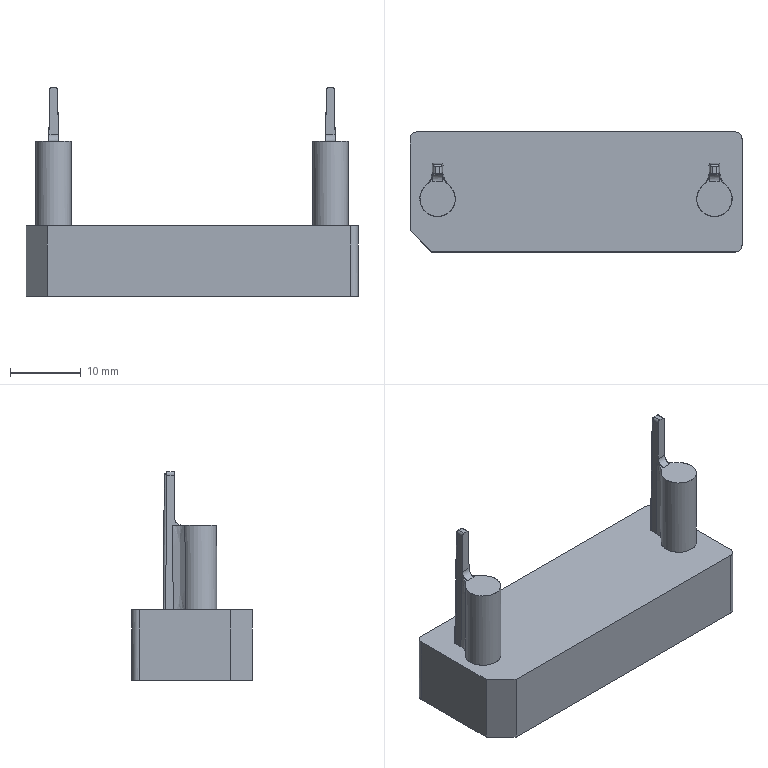NC program | PowerMill | posted with a generic post | part box 47 x 17 x 29.578 mm
Lines 1 to 1019 of 293638:
%
O0001
N104 ( POWERMILL CB  : 2026004.0)
N105 ( POST VER      : 2026.0.0.5161)
N106 ( OPTION FILE   : FANUC)
N107 ( OUTPUT WORKPLANE : WORLD)
N108 (  )
N109 ( TOOL LIST )
N110 (---------------------------------------)
N111 ( NO. | ID        | DIA.| TIP RAD|LENGTH)
N112 (---------------------------------------)
N113 (    1|D10C_1_1_1 |10.0 |  0.0   |85.04 )
N114 (    3|D10_1_1_1  |10.0 |  0.0   |84.72 )
N115 (   14|D4_1_1     | 4.0 |  0.0   |74.72 )
N116 (   13|TEXT_D4_1_1| 4.0 |  0.3   |74.84 )
N117 (---------------------------------------)
N118 (  )
N119 ( NUMBER OF TOOLPATHS: 8.0 )
N120 ( ESTIMATED PROGRAM DURATION: 0 HOURS 18 MIN 45 SEC)
N121 (  )
N122 G00 G21 G80 G40 G17
N123 G90
N124 G54
N125 G53 Z0.0
N126 (---------------)
N127 ( START TOOLPATH : 精公开粗01-扫面平行-D10C )
N128 (---------------)
N129 ( TOOL NO.    :1 )
N130 ( TOOL TYPE   : ENDMILL)
N131 ( TOOL ID     : D10C_1_1_1)
N132 ( TOOL DIA    : 10.0 LENGTH 85.04)
N133 T1
N134 M6
N135 S8000 M03
N136 G00 G90 X0.0 Y0.0
N137 G43 Z10.2 H1
N138
N139 G05 P10000 R4
N140 X31.28 Y11.28
N141 Z1.128
N142 G01 Z-0.072 F6000.0
N143 X26.28 F10000.0
N144 X-26.28
N145 Y5.64
N146 X26.28
N147 Y0.0
N148 X-26.28
N149 Y-5.64
N150 X26.28
N151 Y-11.28
N152 X-26.28
N153 X-31.28
N154 G00 Z10.2
N155 G05 P0
N156 (---------------)
N157 ( END TOOLPATH : 精公开粗01-扫面平行-D10C )
N158 (---------------)
N159 ( START TOOLPATH : 精公开粗01-外形偏置-D10C )
N160 (---------------)
N161 G00 X0.0005 Y0.2935 Z9.878
N162 G05 P10000 R4
N163 X-24.6783 Y17.142
N164 Z0.6807
N165 G01 Z-0.5193 F6000.0
N166 Y16.6145 F10000.0
N167 G03 X-19.9308 Y11.867 I4.7475 J0.0
N168 G01 X18.9125
N169 X18.9494 Y9.1489
N170 X19.7229 Y9.1594
N171 X20.4963 Y9.1274
N172 X21.2697 Y8.9876
N173 X21.8667 Y8.8012
N174 X22.8166 Y8.3298
N175 X23.2599 Y8.0278
N176 X24.3089 Y7.2543
N177 X25.0598 Y6.4809
N178 X25.598 Y5.7075
N179 X25.9103 Y5.1056
N180 X26.2485 Y4.1606
N181 X26.4047 Y3.3872
N182 X26.4674 Y2.6138
N183 X26.4326 Y1.8404
N184 X26.2986 Y1.0669
N185 X26.0623 Y0.2935
N186 X25.7072 Y-0.4799
N187 X25.2095 Y-1.2534
N188 X24.5219 Y-2.0268
N189 X24.3634 Y-2.1726
N190 X23.59 Y-2.7618
N191 X22.8166 Y-3.1839
N192 X22.0432 Y-3.4808
N193 X21.717 Y-3.5736
N194 X21.2697 Y-3.6684
N195 X20.4963 Y-3.7537
N196 X18.9494 Y-3.7612
N197 X18.176 Y-3.705
N198 X17.4771 Y-3.5736
N199 X16.6292 Y-3.2945
N200 X15.8557 Y-2.9141
N201 X15.0823 Y-2.384
N202 X14.6735 Y-2.0268
N203 X14.3089 Y-1.6482
N204 X13.9857 Y-1.2534
N205 X13.5355 Y-0.5653
N206 X13.1325 Y0.2935
N207 X12.8982 Y1.0669
N208 X12.7621 Y1.8404
N209 X12.73 Y2.6138
N210 X12.762 Y3.1936
N211 X12.9446 Y4.1606
N212 X13.2102 Y4.9341
N213 X13.5355 Y5.5996
N214 X14.1354 Y6.4809
N215 X14.3089 Y6.6843
N216 X14.8839 Y7.2543
N217 X15.8557 Y7.9664
N218 X16.6292 Y8.4756
N219 X17.3296 Y8.8012
N220 X18.176 Y9.0437
N221 X18.9494 Y9.1489
N222 X18.9125 Y11.867
N223 X28.876
N224 G02 X29.876 Y10.867 I0.0 J-1.0
N225 G01 Y-10.28
N226 G02 X28.876 Y-11.28 I-1.0 J0.0
N227 G01 X-0.0003
N228 Y-5.7482
N229 Y-1.2482
N230 Y-5.7482
N231 X-7.0067
N232 G02 X-8.6413 Y-3.3411 I0.0 J1.7585
N233 G01 X-8.0409 Y-1.828
N234 G03 X-7.2538 Y1.4975 I-10.9674 J4.3518
N235 G01 X-7.0075 Y4.3174
N236 G02 X-5.0148 Y6.1434 I1.9924 J-0.174
N237 G01 X5.0174 Y6.142
N238 G02 X7.0096 Y4.316 I-0.0003 J-2.0
N239 G01 X7.2551 Y1.5046
N240 X7.3326 Y0.8357
N241 G03 X8.0425 Y-1.8483 I11.4967 J1.605
N242 G01 X8.6372 Y-3.3438
N243 G02 X7.0057 Y-5.7482 I-1.6315 J-0.6487
N244 G01 X-0.0003
N245 Y-11.28
N246 X-28.875
N247 G02 X-29.875 Y-10.28 I0.0 J1.0
N248 G01 Y10.867
N249 G02 X-28.875 Y11.867 I1.0 J0.0
N250 G01 X-19.9308
N251 X-19.8186 Y9.1556
N252 X-19.7219 Y9.1596
N253 X-18.9484 Y9.1488
N254 X-18.175 Y9.0435
N255 X-17.4016 Y8.8278
N256 X-16.6282 Y8.4734
N257 X-15.9364 Y8.0278
N258 X-15.0813 Y7.4198
N259 X-14.8854 Y7.2543
N260 X-14.3079 Y6.6824
N261 X-14.1379 Y6.4809
N262 X-13.5973 Y5.7075
N263 X-13.2095 Y4.9341
N264 X-12.9452 Y4.1606
N265 X-12.7887 Y3.3872
N266 X-12.7281 Y2.6138
N267 X-12.761 Y1.8556
N268 X-12.8958 Y1.0669
N269 X-13.1344 Y0.2935
N270 X-13.4885 Y-0.4799
N271 X-13.9853 Y-1.2534
N272 X-14.3079 Y-1.647
N273 X-14.6711 Y-2.0268
N274 X-15.0813 Y-2.3828
N275 X-15.8547 Y-2.914
N276 X-16.6282 Y-3.2937
N277 X-17.4773 Y-3.5736
N278 X-18.175 Y-3.7049
N279 X-18.9484 Y-3.7612
N280 X-20.4953 Y-3.7536
N281 X-21.2687 Y-3.6685
N282 X-22.0422 Y-3.4814
N283 X-22.8156 Y-3.1841
N284 X-23.529 Y-2.8002
N285 X-24.3624 Y-2.1742
N286 X-24.5226 Y-2.0268
N287 X-25.1359 Y-1.3505
N288 X-25.7049 Y-0.4799
N289 X-25.9093 Y-0.0719
N290 X-26.0593 Y0.2935
N291 X-26.2992 Y1.0669
N292 X-26.4325 Y1.8404
N293 X-26.4672 Y2.6138
N294 X-26.4054 Y3.3872
N295 X-26.2494 Y4.1606
N296 X-25.9849 Y4.9341
N297 X-25.5976 Y5.7075
N298 X-25.1359 Y6.3854
N299 X-24.3624 Y7.2068
N300 X-23.589 Y7.7966
N301 X-22.8156 Y8.3304
N302 X-22.0422 Y8.7297
N303 X-21.2687 Y8.9878
N304 X-20.4953 Y9.1276
N305 X-19.8186 Y9.1556
N306 X-19.9308 Y11.867
N307 G00 Z3.2835
N308 G01 X-24.6783 Y17.142
N309 G00 Z0.2835
N310 G01 Z-0.9165 F6000.0
N311 Y16.6145 F10000.0
N312 G03 X-19.9308 Y11.867 I4.7475 J0.0
N313 G01 X18.9283
N314 X18.9494 Y10.1906
N315 X19.7229 Y10.2004
N316 X20.4963 Y10.1715
N317 X21.2697 Y10.0522
N318 X22.0432 Y9.8331
N319 X22.7013 Y9.5746
N320 X23.59 Y9.0701
N321 X23.9597 Y8.8012
N322 X24.3634 Y8.4517
N323 X24.7766 Y8.0278
N324 X25.1369 Y7.6003
N325 X25.3849 Y7.2543
N326 X25.8286 Y6.4809
N327 X26.1399 Y5.7075
N328 X26.343 Y4.9341
N329 X26.4567 Y4.1606
N330 X26.4795 Y2.6138
N331 X26.4404 Y1.8404
N332 X26.3081 Y1.0669
N333 X26.0718 Y0.2935
N334 X25.7178 Y-0.4799
N335 X25.2226 Y-1.2534
N336 X24.5368 Y-2.0268
N337 X24.3634 Y-2.1853
N338 X23.59 Y-2.7702
N339 X22.8166 Y-3.1942
N340 X22.0432 Y-3.4891
N341 X21.7412 Y-3.5736
N342 X21.2697 Y-3.6734
N343 X20.4963 Y-3.7592
N344 X18.9494 Y-3.766
N345 X18.176 Y-3.7123
N346 X17.4537 Y-3.5736
N347 X16.6292 Y-3.3023
N348 X15.8557 Y-2.9231
N349 X15.0823 Y-2.3964
N350 X14.6591 Y-2.0268
N351 X14.3089 Y-1.6659
N352 X13.9722 Y-1.2534
N353 X13.5355 Y-0.5892
N354 X13.1231 Y0.2935
N355 X12.8855 Y1.0669
N356 X12.762 Y1.7549
N357 X12.717 Y2.6138
N358 X12.7421 Y4.1606
N359 X12.8535 Y4.9341
N360 X13.0533 Y5.7075
N361 X13.3687 Y6.4809
N362 X13.5355 Y6.8053
N363 X13.8102 Y7.2543
N364 X14.3089 Y7.9057
N365 X15.0823 Y8.6753
N366 X15.8557 Y9.2314
N367 X16.4942 Y9.5746
N368 X17.4026 Y9.914
N369 X18.176 Y10.1004
N370 X18.9494 Y10.1906
N371 X18.9283 Y11.867
N372 X28.876
N373 G02 X29.876 Y10.867 I0.0 J-1.0
N374 G01 Y-10.28
N375 G02 X28.876 Y-11.28 I-1.0 J0.0
N376 G01 X0.0635
N377 Y-5.7482
N378 Y-1.2482
N379 Y-5.7482
N380 X-6.9935
N381 G02 X-8.6178 Y-3.3106 I0.0 J1.76
N382 G01 X-7.9525 Y-1.7155
N383 G03 X-6.8547 Y3.557 I-13.1644 J5.4915
N384 G01 X-6.8461 Y4.1159
N385 G02 X-4.8431 Y6.0852 I1.9998 J-0.0307
N386 G01 X4.8771 Y6.0695
N387 G02 X6.8567 Y4.3307 I-0.0033 J-2.0
N388 G01 X7.3245 Y0.7793
N389 X7.3933 Y0.3851
N390 G03 X8.0306 Y-1.8468 I11.4499 J2.0627
N391 G01 X8.6248 Y-3.3429
N392 G02 X6.9921 Y-5.7482 I-1.6327 J-0.6485
N393 G01 X0.0635
N394 Y-11.28
N395 X-28.875
N396 G02 X-29.875 Y-10.28 I0.0 J1.0
N397 G01 Y10.867
N398 G02 X-28.875 Y11.867 I1.0 J0.0
N399 G01 X-20.0744
N400 X-20.0119 Y10.1896
N401 X-19.7219 Y10.2004
N402 X-18.9484 Y10.1906
N403 X-18.175 Y10.1003
N404 X-17.4016 Y9.9165
N405 X-16.6282 Y9.6361
N406 X-15.8547 Y9.231
N407 X-15.2359 Y8.8012
N408 X-14.4185 Y8.0278
N409 X-13.8101 Y7.2543
N410 X-13.5345 Y6.8035
N411 X-13.369 Y6.4809
N412 X-13.0556 Y5.7075
N413 X-12.8535 Y4.9341
N414 X-12.7412 Y4.1606
N415 X-12.7187 Y2.6138
N416 X-12.7519 Y1.8404
N417 X-12.8877 Y1.0669
N418 X-13.1232 Y0.2935
N419 X-13.4768 Y-0.4799
N420 X-13.9712 Y-1.2534
N421 X-14.3079 Y-1.6643
N422 X-14.6585 Y-2.0268
N423 X-15.0813 Y-2.3959
N424 X-15.8547 Y-2.9224
N425 X-16.6282 Y-3.302
N426 X-17.4537 Y-3.5736
N427 X-18.175 Y-3.7122
N428 X-18.9484 Y-3.766
N429 X-20.4953 Y-3.7593
N430 X-21.2687 Y-3.6736
N431 X-22.0422 Y-3.4892
N432 X-22.8156 Y-3.1947
N433 X-23.5441 Y-2.8002
N434 X-24.3624 Y-2.1859
N435 X-24.5355 Y-2.0268
N436 X-25.1359 Y-1.3656
N437 X-25.7189 Y-0.4799
N438 X-25.8641 Y-0.162
N439 X-25.9092 Y-0.0719
N440 X-25.9446 Y0.0143
N441 X-26.0722 Y0.2935
N442 X-26.3077 Y1.0669
N443 X-26.4396 Y1.8404
N444 X-26.4792 Y2.6138
N445 X-26.4562 Y4.1606
N446 X-26.3413 Y4.9341
N447 X-26.1407 Y5.7075
N448 X-25.9093 Y6.3076
N449 X-25.3849 Y7.2543
N450 X-25.1359 Y7.6016
N451 X-24.7766 Y8.0278
N452 X-24.3624 Y8.4529
N453 X-23.9593 Y8.8012
N454 X-23.589 Y9.0717
N455 X-22.8156 Y9.5194
N456 X-22.0422 Y9.8335
N457 X-21.2687 Y10.052
N458 X-20.4953 Y10.1716
N459 X-20.0119 Y10.1896
N460 X-20.0744 Y11.867
N461 X-19.9308
N462 G00 Z2.8862
N463 G01 X-24.6783 Y17.142
N464 G00 Z-0.1138
N465 G01 Z-1.3138 F6000.0
N466 Y16.6145 F10000.0
N467 G03 X-19.9308 Y11.867 I4.7475 J0.0
N468 G01 X18.9294
N469 X18.9494 Y10.1975
N470 X19.7229 Y10.2068
N471 X20.4963 Y10.1788
N472 X21.2697 Y10.0565
N473 X22.0432 Y9.8391
N474 X22.7116 Y9.5746
N475 X23.59 Y9.0779
N476 X23.9676 Y8.8012
N477 X24.3634 Y8.46
N478 X24.7825 Y8.0278
N479 X25.1369 Y7.6027
N480 X25.3892 Y7.2543
N481 X25.8337 Y6.4809
N482 X26.1458 Y5.7075
N483 X26.3471 Y4.9341
N484 X26.4572 Y4.1606
N485 X26.4816 Y2.6138
N486 X26.4457 Y1.8404
N487 X26.3135 Y1.0669
N488 X26.0773 Y0.2935
N489 X25.724 Y-0.4799
N490 X25.2288 Y-1.2534
N491 X24.5436 Y-2.0268
N492 X24.3634 Y-2.1926
N493 X23.59 Y-2.7771
N494 X22.8166 Y-3.1993
N495 X22.0432 Y-3.4936
N496 X21.7579 Y-3.5736
N497 X21.2697 Y-3.6782
N498 X20.4963 Y-3.7628
N499 X18.9494 Y-3.7695
N500 X18.176 Y-3.7163
N501 X17.4026 Y-3.5649
N502 X16.6292 Y-3.3076
N503 X15.8557 Y-2.9297
N504 X15.0823 Y-2.4031
N505 X14.6514 Y-2.0268
N506 X14.3089 Y-1.6725
N507 X13.9662 Y-1.2534
N508 X13.5355 Y-0.5964
N509 X13.1177 Y0.2935
N510 X12.8815 Y1.0669
N511 X12.762 Y1.7311
N512 X12.7134 Y2.6138
N513 X12.7396 Y4.1606
N514 X12.8486 Y4.9341
N515 X13.0487 Y5.7075
N516 X13.3613 Y6.4809
N517 X13.5355 Y6.8148
N518 X13.8058 Y7.2543
N519 X14.3089 Y7.9072
N520 X15.0823 Y8.6827
N521 X15.8557 Y9.2391
N522 X16.4833 Y9.5746
N523 X17.4026 Y9.917
N524 X18.176 Y10.1063
N525 X18.9494 Y10.1975
N526 X18.9294 Y11.867
N527 X28.876
N528 G02 X29.876 Y10.867 I0.0 J-1.0
N529 G01 Y-10.28
N530 G02 X28.876 Y-11.28 I-1.0 J0.0
N531 G01 X0.0767
N532 Y-5.7482
N533 Y-1.2482
N534 Y-5.7482
N535 X-6.9879
N536 G02 X-8.6123 Y-3.311 I0.0 J1.7599
N537 G01 X-7.947 Y-1.7154
N538 G03 X-6.8509 Y3.5558 I-13.1559 J5.4854
N539 G01 X-6.8425 Y4.1144
N540 G02 X-4.8443 Y6.0844 I1.9998 J-0.03
N541 G01 X4.8279 Y6.092
N542 G02 X6.8091 Y4.3765 I0.0016 J-2.0
N543 G01 X7.2607 Y1.2342
N544 G03 X8.0563 Y-1.7615 I13.1524 J1.8899
N545 G01 X8.6645 Y-3.2997
N546 G02 X6.9998 Y-5.7481 I-1.6647 J-0.6583
N547 G01 X0.0767 Y-5.7482
N548 Y-11.28
N549 X-28.875
N550 G02 X-29.875 Y-10.28 I0.0 J1.0
N551 G01 Y10.867
N552 G02 X-28.875 Y11.867 I1.0 J0.0
N553 G01 X-20.0721
N554 X-20.0119 Y10.1963
N555 X-19.7219 Y10.2068
N556 X-18.9484 Y10.1974
N557 X-18.175 Y10.1061
N558 X-17.4016 Y9.9209
N559 X-16.6282 Y9.6411
N560 X-15.8547 Y9.2385
N561 X-15.2274 Y8.8012
N562 X-14.4125 Y8.0278
N563 X-13.8058 Y7.2543
N564 X-13.5345 Y6.813
N565 X-13.3613 Y6.4809
N566 X-13.0491 Y5.7075
N567 X-12.8486 Y4.9341
N568 X-12.7393 Y4.1606
N569 X-12.7134 Y2.6138
N570 X-12.7493 Y1.8404
N571 X-12.8815 Y1.0669
N572 X-13.1179 Y0.2935
N573 X-13.471 Y-0.4799
N574 X-13.9658 Y-1.2534
N575 X-14.3079 Y-1.6712
N576 X-14.6514 Y-2.0268
N577 X-15.0813 Y-2.4023
N578 X-15.8547 Y-2.9291
N579 X-16.6282 Y-3.3072
N580 X-17.4367 Y-3.5736
N581 X-18.175 Y-3.7161
N582 X-18.9484 Y-3.7695
N583 X-20.4953 Y-3.7628
N584 X-21.2687 Y-3.6784
N585 X-22.0422 Y-3.4939
N586 X-22.8156 Y-3.1998
N587 X-23.5537 Y-2.8002
N588 X-24.3624 Y-2.1935
N589 X-24.5436 Y-2.0268
N590 X-25.1359 Y-1.3744
N591 X-25.724 Y-0.4799
N592 X-26.0773 Y0.2935
N593 X-26.3135 Y1.0669
N594 X-26.4457 Y1.8404
N595 X-26.4819 Y2.6138
N596 X-26.4568 Y4.1606
N597 X-26.347 Y4.9341
N598 X-26.1459 Y5.7075
N599 X-25.9093 Y6.3187
N600 X-25.3892 Y7.2543
N601 X-25.1359 Y7.604
N602 X-24.7825 Y8.0278
N603 X-24.3624 Y8.4609
N604 X-23.9676 Y8.8012
N605 X-23.589 Y9.0786
N606 X-22.8156 Y9.525
N607 X-22.0422 Y9.8394
N608 X-21.2687 Y10.0568
N609 X-20.4953 Y10.1789
N610 X-20.0119 Y10.1963
N611 X-20.0721 Y11.867
N612 X-19.9308
N613 G00 Z2.489
N614 G01 X-24.6783 Y17.142
N615 G00 Z-0.5111
N616 G01 Z-1.7111 F6000.0
N617 Y16.6145 F10000.0
N618 G03 X-19.9308 Y11.867 I4.7475 J0.0
N619 G01 X18.9299
N620 X18.9494 Y10.2012
N621 X19.7229 Y10.2102
N622 X20.4963 Y10.1826
N623 X21.2697 Y10.0608
N624 X22.0432 Y9.844
N625 X22.7225 Y9.5746
N626 X23.59 Y9.0837
N627 X23.9754 Y8.8012
N628 X24.3634 Y8.4667
N629 X24.789 Y8.0278
N630 X25.1369 Y7.6106
N631 X25.395 Y7.2543
N632 X25.8389 Y6.4809
N633 X26.1509 Y5.7075
N634 X26.3512 Y4.9341
N635 X26.4581 Y4.1606
N636 X26.4851 Y2.6138
N637 X26.4496 Y1.8404
N638 X26.3177 Y1.0669
N639 X26.0821 Y0.2935
N640 X25.7293 Y-0.4799
N641 X25.2349 Y-1.2534
N642 X24.5507 Y-2.0268
N643 X24.3634 Y-2.1991
N644 X23.59 Y-2.7828
N645 X22.8166 Y-3.2044
N646 X22.0432 Y-3.4981
N647 X21.7745 Y-3.5736
N648 X21.2697 Y-3.6822
N649 X20.4963 Y-3.7664
N650 X18.9494 Y-3.773
N651 X18.176 Y-3.7202
N652 X17.4197 Y-3.5736
N653 X16.6292 Y-3.3125
N654 X15.8557 Y-2.9351
N655 X15.0823 Y-2.4093
N656 X14.6443 Y-2.0268
N657 X14.3089 Y-1.6796
N658 X13.9601 Y-1.2534
N659 X13.5355 Y-0.6056
N660 X13.1129 Y0.2935
N661 X12.8773 Y1.0669
N662 X12.762 Y1.7008
N663 X12.7099 Y2.6138
N664 X12.7369 Y4.1606
N665 X12.8438 Y4.9341
N666 X13.0441 Y5.7075
N667 X13.3561 Y6.4809
N668 X13.5355 Y6.8243
N669 X13.8 Y7.2543
N670 X14.3089 Y7.9147
N671 X15.0823 Y8.6891
N672 X15.8557 Y9.2447
N673 X16.4724 Y9.5746
N674 X17.4026 Y9.9215
N675 X18.176 Y10.1111
N676 X18.9494 Y10.2012
N677 X18.9299 Y11.867
N678 X28.876
N679 G02 X29.876 Y10.867 I0.0 J-1.0
N680 G01 Y-10.28
N681 G02 X28.876 Y-11.28 I-1.0 J0.0
N682 G01 X0.0643
N683 Y-5.7482
N684 Y-1.2482
N685 Y-5.7482
N686 X-6.9821
N687 G02 X-8.6069 Y-3.311 I0.0 J1.7602
N688 G01 X-7.9418 Y-1.715
N689 G03 X-6.847 Y3.555 I-13.1563 J5.482
N690 G01 X-6.8387 Y4.1136
N691 G02 X-4.8355 Y6.0838 I1.9998 J-0.0298
N692 G01 X4.8707 Y6.0676
N693 G02 X6.8502 Y4.3289 I-0.0034 J-2.0
N694 G01 X7.3257 Y0.7206
N695 X7.3983 Y0.3149
N696 G03 X8.0213 Y-1.8462 I11.4373 J2.1268
N697 G01 X8.6146 Y-3.3427
N698 G02 X6.9808 Y-5.7482 I-1.6338 J-0.6479
N699 G01 X0.0643
N700 Y-11.28
N701 X-28.875
N702 G02 X-29.875 Y-10.28 I0.0 J1.0
N703 G01 Y10.867
N704 G02 X-28.875 Y11.867 I1.0 J0.0
N705 G01 X-20.0713
N706 X-20.0119 Y10.1999
N707 X-19.7219 Y10.2102
N708 X-18.9484 Y10.2011
N709 X-18.175 Y10.111
N710 X-17.4016 Y9.9253
N711 X-16.6282 Y9.6458
N712 X-15.8547 Y9.2441
N713 X-15.2196 Y8.8012
N714 X-14.406 Y8.0278
N715 X-13.8 Y7.2543
N716 X-13.5345 Y6.8225
N717 X-13.3561 Y6.4809
N718 X-13.0441 Y5.7075
N719 X-12.8438 Y4.9341
N720 X-12.7369 Y4.1606
N721 X-12.7099 Y2.6138
N722 X-12.7454 Y1.8404
N723 X-12.8773 Y1.0669
N724 X-13.1129 Y0.2935
N725 X-13.4657 Y-0.4799
N726 X-13.9601 Y-1.2534
N727 X-14.3079 Y-1.6785
N728 X-14.6443 Y-2.0268
N729 X-15.0813 Y-2.4085
N730 X-15.8547 Y-2.9346
N731 X-16.6282 Y-3.3121
N732 X-17.4197 Y-3.5736
N733 X-18.175 Y-3.7201
N734 X-18.9484 Y-3.773
N735 X-20.4953 Y-3.7664
N736 X-21.2687 Y-3.6824
N737 X-22.0422 Y-3.4984
N738 X-22.8156 Y-3.2049
N739 X-23.589 Y-2.7835
N740 X-24.3624 Y-2.2
N741 X-24.5507 Y-2.0268
N742 X-25.1359 Y-1.3823
N743 X-25.7293 Y-0.4799
N744 X-26.0821 Y0.2935
N745 X-26.3177 Y1.0669
N746 X-26.4496 Y1.8404
N747 X-26.4851 Y2.6138
N748 X-26.4581 Y4.1606
N749 X-26.3512 Y4.9341
N750 X-26.1509 Y5.7075
N751 X-25.9093 Y6.3297
N752 X-25.395 Y7.2543
N753 X-25.1359 Y7.6119
N754 X-24.789 Y8.0278
N755 X-24.3624 Y8.4677
N756 X-23.9754 Y8.8012
N757 X-23.589 Y9.0844
N758 X-22.8156 Y9.5304
N759 X-22.0422 Y9.8443
N760 X-21.2687 Y10.061
N761 X-20.4953 Y10.1827
N762 X-20.0119 Y10.1999
N763 X-20.0713 Y11.867
N764 X-19.9308
N765 G00 Z2.0917
N766 G01 X-24.6783 Y17.142
N767 G00 Z-0.9083
N768 G01 Z-2.1083 F6000.0
N769 Y16.6145 F10000.0
N770 G03 X-19.9308 Y11.867 I4.7475 J0.0
N771 G01 X18.9303
N772 X18.9494 Y10.2048
N773 X19.7229 Y10.2137
N774 X20.4963 Y10.1864
N775 X21.2697 Y10.065
N776 X22.0432 Y9.8486
N777 X22.7333 Y9.5746
N778 X23.59 Y9.0895
N779 X23.9832 Y8.8012
N780 X24.3634 Y8.4734
N781 X24.7955 Y8.0278
N782 X25.1369 Y7.6185
N783 X25.4008 Y7.2543
N784 X25.844 Y6.4809
N785 X26.1555 Y5.7075
N786 X26.3553 Y4.9341
N787 X26.4618 Y4.1606
N788 X26.4885 Y2.6138
N789 X26.4534 Y1.8404
N790 X26.322 Y1.0669
N791 X26.0869 Y0.2935
N792 X25.7347 Y-0.4799
N793 X25.241 Y-1.2534
N794 X24.5578 Y-2.0268
N795 X24.3634 Y-2.2057
N796 X23.59 Y-2.7885
N797 X22.8166 Y-3.2094
N798 X22.0432 Y-3.5027
N799 X21.7912 Y-3.5736
N800 X21.2697 Y-3.6863
N801 X20.4963 Y-3.77
N802 X18.9494 Y-3.7765
N803 X18.176 Y-3.7241
N804 X17.4027 Y-3.5736
N805 X16.6292 Y-3.3174
N806 X15.8557 Y-2.9406
N807 X15.0823 Y-2.4156
N808 X14.6372 Y-2.0268
N809 X14.3089 Y-1.6869
N810 X13.954 Y-1.2534
N811 X13.5355 Y-0.6151
N812 X13.1081 Y0.2935
N813 X12.873 Y1.0669
N814 X12.762 Y1.6706
N815 X12.7065 Y2.6138
N816 X12.7332 Y4.1606
N817 X12.8397 Y4.9341
N818 X13.0395 Y5.7075
N819 X13.351 Y6.4809
N820 X13.5355 Y6.8338
N821 X13.7942 Y7.2543
N822 X14.3089 Y7.9223
N823 X15.0823 Y8.6955
N824 X15.8557 Y9.2503
N825 X16.4616 Y9.5746
N826 X17.4026 Y9.926
N827 X18.176 Y10.1152
N828 X18.9494 Y10.2048
N829 X18.9303 Y11.867
N830 X28.876
N831 G02 X29.876 Y10.867 I0.0 J-1.0
N832 G01 Y-10.28
N833 G02 X28.876 Y-11.28 I-1.0 J0.0
N834 G01 X0.0773
N835 Y-5.7482
N836 Y-1.2482
N837 Y-5.7482
N838 X-6.9761
N839 G02 X-8.6014 Y-3.3111 I0.0 J1.7605
N840 G01 X-7.9365 Y-1.714
N841 G03 X-6.8431 Y3.5545 I-13.1615 J5.4793
N842 G01 X-6.8348 Y4.1132
N843 G02 X-4.8367 Y6.0837 I1.9998 J-0.0295
N844 G01 X4.8196 Y6.0916
N845 G02 X6.8008 Y4.3765 I0.0016 J-2.0
N846 G01 X7.2536 Y1.2307
N847 G03 X8.0471 Y-1.7594 I13.1769 J1.8965
N848 G01 X8.6546 Y-3.299
N849 G02 X6.9882 Y-5.7481 I-1.6665 J-0.6576
N850 G01 X0.0773 Y-5.7482
N851 Y-11.28
N852 X-28.875
N853 G02 X-29.875 Y-10.28 I0.0 J1.0
N854 G01 Y10.867
N855 G02 X-28.875 Y11.867 I1.0 J0.0
N856 G01 X-20.0705
N857 X-20.0119 Y10.2035
N858 X-19.7219 Y10.2137
N859 X-18.9484 Y10.2047
N860 X-18.175 Y10.1151
N861 X-17.4016 Y9.9297
N862 X-16.6282 Y9.6502
N863 X-15.8547 Y9.2496
N864 X-15.2118 Y8.8012
N865 X-14.3995 Y8.0278
N866 X-13.7942 Y7.2543
N867 X-13.5345 Y6.832
N868 X-13.351 Y6.4809
N869 X-13.0395 Y5.7075
N870 X-12.8397 Y4.9341
N871 X-12.7332 Y4.1606
N872 X-12.7065 Y2.6138
N873 X-12.7416 Y1.8404
N874 X-12.873 Y1.0669
N875 X-13.1081 Y0.2935
N876 X-13.4603 Y-0.4799
N877 X-13.954 Y-1.2534
N878 X-14.3079 Y-1.6858
N879 X-14.6372 Y-2.0268
N880 X-15.0813 Y-2.4148
N881 X-15.8547 Y-2.94
N882 X-16.6282 Y-3.317
N883 X-17.4027 Y-3.5736
N884 X-18.175 Y-3.724
N885 X-18.9484 Y-3.7765
N886 X-20.4953 Y-3.7701
N887 X-21.2687 Y-3.6865
N888 X-22.0422 Y-3.503
N889 X-22.8156 Y-3.2099
N890 X-23.5716 Y-2.8002
N891 X-24.3624 Y-2.2065
N892 X-24.5578 Y-2.0268
N893 X-25.1359 Y-1.3902
N894 X-25.7347 Y-0.4799
N895 X-26.0869 Y0.2935
N896 X-26.322 Y1.0669
N897 X-26.4534 Y1.8404
N898 X-26.4885 Y2.6138
N899 X-26.4618 Y4.1606
N900 X-26.3553 Y4.9341
N901 X-26.1555 Y5.7075
N902 X-25.9093 Y6.3407
N903 X-25.4008 Y7.2543
N904 X-25.1359 Y7.6198
N905 X-24.7955 Y8.0278
N906 X-24.3624 Y8.4744
N907 X-23.9832 Y8.8012
N908 X-23.589 Y9.0902
N909 X-22.8156 Y9.5356
N910 X-22.0422 Y9.8489
N911 X-21.2687 Y10.0652
N912 X-20.4953 Y10.1865
N913 X-20.0119 Y10.2035
N914 X-20.0705 Y11.867
N915 X-19.9308
N916 G00 Z1.6944
N917 G01 X-24.6783 Y17.142
N918 G00 Z-1.3056
N919 G01 Z-2.5056 F6000.0
N920 Y16.6145 F10000.0
N921 G03 X-19.9308 Y11.867 I4.7475 J0.0
N922 G01 X18.9307
N923 X18.9494 Y10.2085
N924 X19.7229 Y10.2172
N925 X20.4963 Y10.1902
N926 X21.2697 Y10.0692
N927 X22.0432 Y9.8532
N928 X22.7442 Y9.5746
N929 X23.59 Y9.0953
N930 X23.9911 Y8.8012
N931 X24.3634 Y8.4801
N932 X24.802 Y8.0278
N933 X25.1369 Y7.6264
N934 X25.4066 Y7.2543
N935 X25.8491 Y6.4809
N936 X26.1601 Y5.7075
N937 X26.3594 Y4.9341
N938 X26.4656 Y4.1606
N939 X26.492 Y2.6138
N940 X26.4573 Y1.8404
N941 X26.3263 Y1.0669
N942 X26.0916 Y0.2935
N943 X25.74 Y-0.4799
N944 X25.247 Y-1.2534
N945 X24.5649 Y-2.0268
N946 X24.3634 Y-2.2122
N947 X23.59 Y-2.7942
N948 X22.8166 Y-3.2145
N949 X22.0432 Y-3.5072
N950 X21.8079 Y-3.5736
N951 X21.2697 Y-3.6904
N952 X20.4963 Y-3.7736
N953 X18.9494 Y-3.78
N954 X18.176 Y-3.728
N955 X17.4026 Y-3.578
N956 X16.6292 Y-3.3223
N957 X15.8557 Y-2.9461
N958 X15.0823 Y-2.4218
N959 X14.6301 Y-2.0268
N960 X14.3089 Y-1.6942
N961 X13.948 Y-1.2534
N962 X13.5355 Y-0.6245
N963 X13.1034 Y0.2935
N964 X12.8687 Y1.0669
N965 X12.762 Y1.6413
N966 X12.703 Y2.6138
N967 X12.7294 Y4.1606
N968 X12.8356 Y4.9341
N969 X13.0349 Y5.7075
N970 X13.3459 Y6.4809
N971 X13.5355 Y6.8433
N972 X13.7884 Y7.2543
N973 X14.3089 Y7.9299
N974 X15.0823 Y8.7019
N975 X15.8557 Y9.2558
N976 X16.4507 Y9.5746
N977 X17.4026 Y9.9305
N978 X18.176 Y10.1193
N979 X18.9494 Y10.2085
N980 X18.9307 Y11.867
N981 X28.876
N982 G02 X29.876 Y10.867 I0.0 J-1.0
N983 G01 Y-10.28
N984 G02 X28.876 Y-11.28 I-1.0 J0.0
N985 G01 X0.0774
N986 Y-5.7482
N987 Y-1.2482
N988 Y-5.7482
N989 X-6.9702
N990 G02 X-8.5959 Y-3.3112 I0.0 J1.7608
N991 G01 X-7.9311 Y-1.7129
N992 G03 X-6.8392 Y3.5541 I-13.1668 J5.4764
N993 G01 X-6.831 Y4.1129
N994 G02 X-4.8329 Y6.0835 I1.9998 J-0.0294
N995 G01 X4.8155 Y6.0916
N996 G02 X6.7968 Y4.3764 I0.0016 J-2.0
N997 G01 X7.2495 Y1.2299
N998 G03 X8.0421 Y-1.7588 I13.1831 J1.8969
N999 G01 X8.6493 Y-3.2988
N1000 G02 X6.9822 Y-5.7481 I-1.6671 J-0.6573
N1001 G01 X0.0774 Y-5.7482
N1002 Y-11.28
N1003 X-28.875
N1004 G02 X-29.875 Y-10.28 I0.0 J1.0
N1005 G01 Y10.867
N1006 G02 X-28.875 Y11.867 I1.0 J0.0
N1007 G01 X-20.0696
N1008 X-20.0119 Y10.2071
N1009 X-19.7219 Y10.2172
N1010 X-18.9484 Y10.2084
N1011 X-18.175 Y10.1191
N1012 X-17.4016 Y9.9341
N1013 X-16.6282 Y9.6548
N1014 X-15.8547 Y9.2552
N1015 X-15.2039 Y8.8012
N1016 X-14.393 Y8.0278
N1017 X-13.7884 Y7.2543
N1018 X-13.5345 Y6.8415
N1019 X-13.3459 Y6.4809
N1020 X-13.0349 Y5.7075
N1021 X-12.8356 Y4.9341
N1022 X-12.7294 Y4.1606
N1023 X-12.703 Y2.6138
N1024 X-12.7377 Y1.8404
N1025 X-12.8687 Y1.0669
N1026 X-13.1034 Y0.2935
N1027 X-13.455 Y-0.4799
N1028 X-13.948 Y-1.2534
N1029 X-14.3079 Y-1.6931
N1030 X-14.6301 Y-2.0268
N1031 X-15.0813 Y-2.421
N1032 X-15.8547 Y-2.9455
N1033 X-16.6282 Y-3.3219
N1034 X-17.3864 Y-3.5736
N1035 X-18.175 Y-3.7279
N1036 X-18.9484 Y-3.78
N1037 X-20.4953 Y-3.7737
N1038 X-21.2687 Y-3.6905
N1039 X-22.0422 Y-3.5075
N1040 X-22.8156 Y-3.215
N1041 X-23.5805 Y-2.8002
N1042 X-24.3624 Y-2.2131
N1043 X-24.5649 Y-2.0268
N1044 X-25.1359 Y-1.398
N1045 X-25.74 Y-0.4799
N1046 X-26.0916 Y0.2935
N1047 X-26.3263 Y1.0669
N1048 X-26.4573 Y1.8404
N1049 X-26.492 Y2.6138
N1050 X-26.4656 Y4.1606
N1051 X-26.3594 Y4.9341
N1052 X-26.1601 Y5.7075
N1053 X-25.9093 Y6.3517
N1054 X-25.4066 Y7.2543
N1055 X-25.1359 Y7.6277
N1056 X-24.802 Y8.0278
N1057 X-24.3624 Y8.4811
N1058 X-23.9911 Y8.8012
N1059 X-23.589 Y9.096
N1060 X-22.8156 Y9.5407
N1061 X-22.0422 Y9.8535
N1062 X-21.2687 Y10.0695
N1063 X-20.4953 Y10.1903
N1064 X-20.0119 Y10.2071
N1065 X-20.0696 Y11.867
N1066 X-19.9308
N1067 G00 Z1.2972
N1068 G01 X-24.6783 Y17.142
N1069 G00 Z-1.7028
N1070 G01 Z-2.9028 F6000.0
N1071 Y16.6145 F10000.0
N1072 G03 X-19.9308 Y11.867 I4.7475 J0.0
N1073 G01 X18.9312
N1074 X18.9494 Y10.2121
N1075 X19.7229 Y10.2206
N1076 X20.4963 Y10.194
N1077 X21.2697 Y10.0735
N1078 X22.0432 Y9.8578
N1079 X22.755 Y9.5746
N1080 X23.59 Y9.1011
N1081 X23.9989 Y8.8012
N1082 X24.3634 Y8.4868
N1083 X24.8085 Y8.0278
N1084 X25.1369 Y7.6343
N1085 X25.4124 Y7.2543
N1086 X25.8543 Y6.4809
N1087 X26.1647 Y5.7075
N1088 X26.3636 Y4.9341
N1089 X26.4694 Y4.1606
N1090 X26.4955 Y2.6138
N1091 X26.4611 Y1.8404
N1092 X26.3306 Y1.0669
N1093 X26.0964 Y0.2935
N1094 X25.7453 Y-0.4799
N1095 X25.2531 Y-1.2534
N1096 X24.5719 Y-2.0268
N1097 X24.3634 Y-2.2187
N1098 X23.59 Y-2.7999
N1099 X22.8166 Y-3.2195
N1100 X22.0432 Y-3.5117
N1101 X21.8246 Y-3.5736
N1102 X21.2697 Y-3.6944
N1103 X20.4963 Y-3.7773
N1104 X18.9494 Y-3.7835
N1105 X18.176 Y-3.7319
N1106 X17.4026 Y-3.5823
N1107 X16.6292 Y-3.3271
N1108 X15.8557 Y-2.9515
N1109 X15.0823 Y-2.428
N1110 X14.6231 Y-2.0268
N1111 X14.3089 Y-1.7016
N1112 X13.9419 Y-1.2534
N1113 X13.5355 Y-0.6339
N1114 X13.0986 Y0.2935
N1115 X12.8644 Y1.0669
N1116 X12.762 Y1.6137